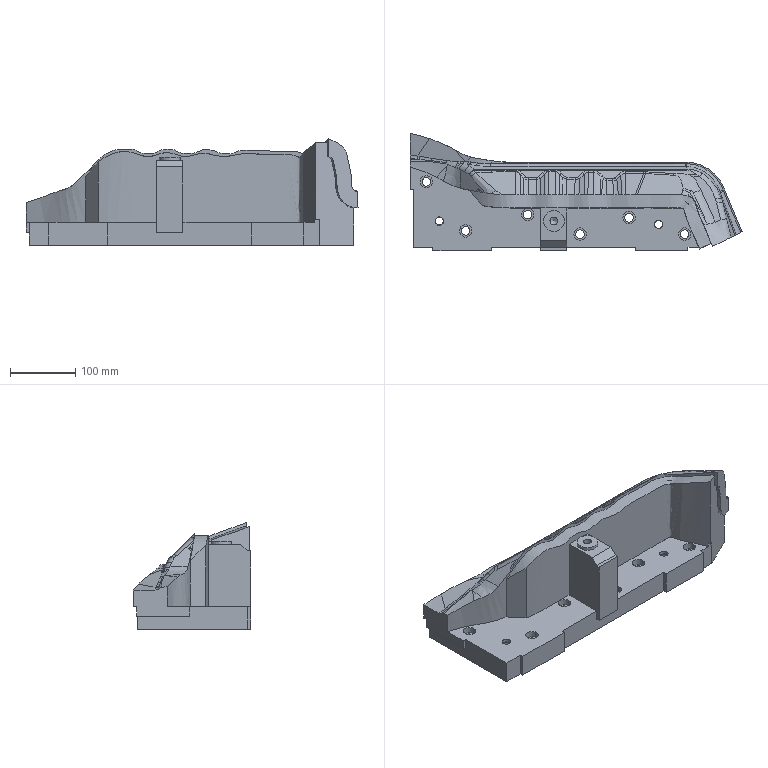Part | NX | features solid 2 | 1 solid | 191 faces | box 507.584 x 178.9 x 163.242 mm | volume 5283274 mm3 | spline 73 | plane 60 | cylinder 57 | cone 1 | commonest cylinder face diameters 20 x16 40 x12 13 x8 19 x6 12 x3 60 x3